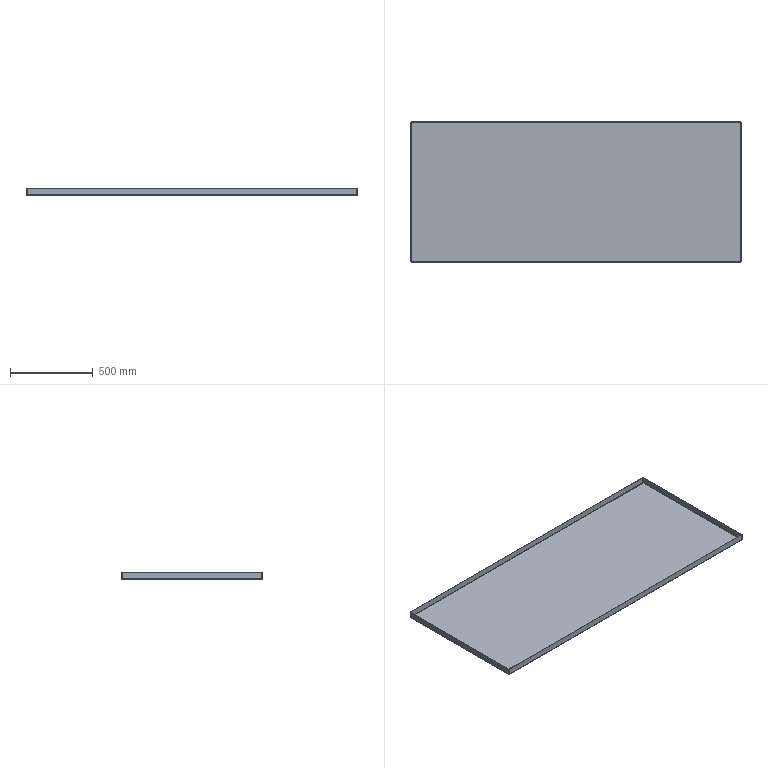Part | SolidWorks | features EdgeFlange 1, FlatPattern 1, SMBaseFlange 1, SheetMetal 1 | 1 solid | 38 faces | box 2000 x 850 x 40 mm | volume 3823030 mm3 | plane 22 | spline 8 | cylinder 8 | commonest cylinder face diameters 1.473 x4 5.473 x4
STEP:
#1=CARTESIAN_POINT('',(997.263,422.263,-2.));
#2=VERTEX_POINT('',#1);
#3=CARTESIAN_POINT('',(997.263,-422.263,-2.));
#4=VERTEX_POINT('',#3);
#5=CARTESIAN_POINT('',(997.263,422.293,-2.));
#6=DIRECTION('',(0.,-1.,0.));
#7=VECTOR('',#6,1000.);
#8=LINE('',#5,#7);
#9=EDGE_CURVE('',#2,#4,#8,.T.);
#10=ORIENTED_EDGE('',*,*,#9,.T.);
#11=CARTESIAN_POINT('',(-997.263,-422.263,-2.));
#12=VERTEX_POINT('',#11);
#13=CARTESIAN_POINT('',(997.293,-422.263,-2.));
#14=DIRECTION('',(-1.,0.,0.));
#15=VECTOR('',#14,1000.);
#16=LINE('',#13,#15);
#17=EDGE_CURVE('',#4,#12,#16,.T.);
#18=ORIENTED_EDGE('',*,*,#17,.T.);
#19=CARTESIAN_POINT('',(-997.263,422.263,-2.));
#20=VERTEX_POINT('',#19);
#21=CARTESIAN_POINT('',(-997.263,-422.293,-2.));
#22=DIRECTION('',(0.,1.,0.));
#23=VECTOR('',#22,1000.);
#24=LINE('',#21,#23);
#25=EDGE_CURVE('',#12,#20,#24,.T.);
#26=ORIENTED_EDGE('',*,*,#25,.T.);
#27=CARTESIAN_POINT('',(-997.293,422.263,-2.));
#28=DIRECTION('',(1.,0.,0.));
#29=VECTOR('',#28,1000.);
#30=LINE('',#27,#29);
#31=EDGE_CURVE('',#20,#2,#30,.T.);
#32=ORIENTED_EDGE('',*,*,#31,.T.);
#33=EDGE_LOOP('',(#10,#18,#26,#32));
#34=FACE_OUTER_BOUND('',#33,.T.);
#35=CARTESIAN_POINT('',(0.,0.,-2.));
#36=DIRECTION('',(0.,0.,-1.));
#37=DIRECTION('',(-1.,0.,0.));
#38=AXIS2_PLACEMENT_3D('',#35,#36,#37);
#39=PLANE('',#38);
#40=ADVANCED_FACE('',(#34),#39,.T.);
#41=CARTESIAN_POINT('',(997.263,-422.263,0.));
#42=VERTEX_POINT('',#41);
#43=CARTESIAN_POINT('',(-997.263,-422.263,0.));
#44=VERTEX_POINT('',#43);
#45=CARTESIAN_POINT('',(997.293,-422.263,0.));
#46=DIRECTION('',(-1.,0.,0.));
#47=VECTOR('',#46,1000.);
#48=LINE('',#45,#47);
#49=EDGE_CURVE('',#42,#44,#48,.T.);
#50=ORIENTED_EDGE('',*,*,#49,.F.);
#51=CARTESIAN_POINT('',(997.263,422.263,0.));
#52=VERTEX_POINT('',#51);
#53=CARTESIAN_POINT('',(997.263,422.293,0.));
#54=DIRECTION('',(0.,-1.,0.));
#55=VECTOR('',#54,1000.);
#56=LINE('',#53,#55);
#57=EDGE_CURVE('',#52,#42,#56,.T.);
#58=ORIENTED_EDGE('',*,*,#57,.F.);
#59=CARTESIAN_POINT('',(-997.263,422.263,0.));
#60=VERTEX_POINT('',#59);
#61=CARTESIAN_POINT('',(-997.293,422.263,0.));
#62=DIRECTION('',(1.,0.,0.));
#63=VECTOR('',#62,1000.);
#64=LINE('',#61,#63);
#65=EDGE_CURVE('',#60,#52,#64,.T.);
#66=ORIENTED_EDGE('',*,*,#65,.F.);
#67=CARTESIAN_POINT('',(-997.263,-422.293,0.));
#68=DIRECTION('',(0.,1.,0.));
#69=VECTOR('',#68,1000.);
#70=LINE('',#67,#69);
#71=EDGE_CURVE('',#44,#60,#70,.T.);
#72=ORIENTED_EDGE('',*,*,#71,.F.);
#73=EDGE_LOOP('',(#50,#58,#66,#72));
#74=FACE_OUTER_BOUND('',#73,.T.);
#75=CARTESIAN_POINT('',(0.,0.,0.));
#76=DIRECTION('',(0.,0.,-1.));
#77=DIRECTION('',(-1.,0.,0.));
#78=AXIS2_PLACEMENT_3D('',#75,#76,#77);
#79=PLANE('',#78);
#80=ADVANCED_FACE('',(#74),#79,.F.);
#81=CARTESIAN_POINT('',(997.293,425.,0.7366));
#82=VERTEX_POINT('',#81);
#83=CARTESIAN_POINT('',(997.293,423.,0.7366));
#84=VERTEX_POINT('',#83);
#85=CARTESIAN_POINT('',(997.293,423.,0.7366));
#86=DIRECTION('',(0.,-1.,0.));
#87=VECTOR('',#86,1000.);
#88=LINE('',#85,#87);
#89=EDGE_CURVE('',#82,#84,#88,.T.);
#90=ORIENTED_EDGE('',*,*,#89,.T.);
#91=CARTESIAN_POINT('',(997.263,422.263,0.));
#92=CARTESIAN_POINT('',(997.268,422.456,0.));
#93=CARTESIAN_POINT('',(997.273,422.648,0.07939));
#94=CARTESIAN_POINT('',(997.283,422.921,0.3521));
#95=CARTESIAN_POINT('',(997.288,423.,0.5438));
#96=CARTESIAN_POINT('',(997.293,423.,0.7366));
#97=B_SPLINE_CURVE_WITH_KNOTS('',3,(#91,#92,#93,#94,#95,#96),.UNSPECIFIED.,.F.,.F.,(4,2,4),(0.,0.5,1.),.UNSPECIFIED.);
#98=EDGE_CURVE('',#52,#84,#97,.T.);
#99=ORIENTED_EDGE('',*,*,#98,.F.);
#100=CARTESIAN_POINT('',(997.263,422.263,0.));
#101=DIRECTION('',(0.,0.,-1.));
#102=VECTOR('',#101,1000.);
#103=LINE('',#100,#102);
#104=EDGE_CURVE('',#52,#2,#103,.T.);
#105=ORIENTED_EDGE('',*,*,#104,.T.);
#106=CARTESIAN_POINT('',(997.263,422.263,-2.));
#107=CARTESIAN_POINT('',(997.266,422.622,-2.));
#108=CARTESIAN_POINT('',(997.268,422.98,-1.929));
#109=CARTESIAN_POINT('',(997.273,423.642,-1.655));
#110=CARTESIAN_POINT('',(997.276,423.945,-1.452));
#111=CARTESIAN_POINT('',(997.281,424.452,-0.9452));
#112=CARTESIAN_POINT('',(997.283,424.655,-0.6416));
#113=CARTESIAN_POINT('',(997.288,424.929,0.0203));
#114=CARTESIAN_POINT('',(997.29,425.,0.3784));
#115=CARTESIAN_POINT('',(997.293,425.,0.7366));
#116=B_SPLINE_CURVE_WITH_KNOTS('',3,(#106,#107,#108,#109,#110,#111,#112,#113,#114,#115),.UNSPECIFIED.,.F.,.F.,(4,2,2,2,4),(0.,0.25,0.5,0.75,1.),.UNSPECIFIED.);
#117=EDGE_CURVE('',#2,#82,#116,.T.);
#118=ORIENTED_EDGE('',*,*,#117,.T.);
#119=EDGE_LOOP('',(#90,#99,#105,#118));
#120=FACE_OUTER_BOUND('',#119,.T.);
#121=CARTESIAN_POINT('',(997.263,422.263,-2.02));
#122=CARTESIAN_POINT('',(997.266,422.624,-2.02));
#123=CARTESIAN_POINT('',(997.268,422.985,-1.948));
#124=CARTESIAN_POINT('',(997.273,423.652,-1.672));
#125=CARTESIAN_POINT('',(997.276,423.957,-1.468));
#126=CARTESIAN_POINT('',(997.281,424.468,-0.9575));
#127=CARTESIAN_POINT('',(997.283,424.672,-0.6517));
#128=CARTESIAN_POINT('',(997.288,424.948,0.01507));
#129=CARTESIAN_POINT('',(997.29,425.02,0.3757));
#130=CARTESIAN_POINT('',(997.293,425.02,0.7366));
#131=CARTESIAN_POINT('',(997.263,422.263,-2.));
#132=CARTESIAN_POINT('',(997.266,422.622,-2.));
#133=CARTESIAN_POINT('',(997.268,422.98,-1.929));
#134=CARTESIAN_POINT('',(997.273,423.642,-1.655));
#135=CARTESIAN_POINT('',(997.276,423.945,-1.452));
#136=CARTESIAN_POINT('',(997.281,424.452,-0.9452));
#137=CARTESIAN_POINT('',(997.283,424.655,-0.6416));
#138=CARTESIAN_POINT('',(997.288,424.929,0.0203));
#139=CARTESIAN_POINT('',(997.29,425.,0.3783));
#140=CARTESIAN_POINT('',(997.293,425.,0.7366));
#141=CARTESIAN_POINT('',(997.263,422.263,0.));
#142=CARTESIAN_POINT('',(997.266,422.36,0.));
#143=CARTESIAN_POINT('',(997.268,422.456,0.01917));
#144=CARTESIAN_POINT('',(997.273,422.634,0.09297));
#145=CARTESIAN_POINT('',(997.276,422.716,0.1476));
#146=CARTESIAN_POINT('',(997.281,422.852,0.2839));
#147=CARTESIAN_POINT('',(997.283,422.907,0.3656));
#148=CARTESIAN_POINT('',(997.288,422.981,0.5438));
#149=CARTESIAN_POINT('',(997.29,423.,0.6402));
#150=CARTESIAN_POINT('',(997.293,423.,0.7366));
#151=CARTESIAN_POINT('',(997.263,422.263,0.0202));
#152=CARTESIAN_POINT('',(997.266,422.357,0.0202));
#153=CARTESIAN_POINT('',(997.268,422.451,0.03885));
#154=CARTESIAN_POINT('',(997.273,422.624,0.1106));
#155=CARTESIAN_POINT('',(997.276,422.704,0.1637));
#156=CARTESIAN_POINT('',(997.281,422.836,0.2963));
#157=CARTESIAN_POINT('',(997.283,422.889,0.3758));
#158=CARTESIAN_POINT('',(997.288,422.961,0.5491));
#159=CARTESIAN_POINT('',(997.29,422.98,0.6428));
#160=CARTESIAN_POINT('',(997.293,422.98,0.7366));
#161=B_SPLINE_SURFACE_WITH_KNOTS('',1,3,((#121,#122,#123,#124,#125,#126,#127,#128,#129,#130),(#131,#132,#133,#134,#135,#136,#137,#138,#139,#140),(#141,#142,#143,#144,#145,#146,#147,#148,#149,#150),(#151,#152,#153,#154,#155,#156,#157,#158,#159,#160)),.UNSPECIFIED.,.F.,.F.,.F.,(2,1,1,2),(4,2,2,2,4),(-0.01,0.,1.,1.01),(0.,0.25,0.5,0.75,1.),.UNSPECIFIED.);
#162=ADVANCED_FACE('',(#120),#161,.F.);
#163=CARTESIAN_POINT('',(-997.293,423.,0.7366));
#164=VERTEX_POINT('',#163);
#165=CARTESIAN_POINT('',(-997.293,423.,0.7366));
#166=CARTESIAN_POINT('',(-997.288,423.,0.5438));
#167=CARTESIAN_POINT('',(-997.283,422.921,0.3521));
#168=CARTESIAN_POINT('',(-997.273,422.648,0.07939));
#169=CARTESIAN_POINT('',(-997.268,422.456,0.));
#170=CARTESIAN_POINT('',(-997.263,422.263,0.));
#171=B_SPLINE_CURVE_WITH_KNOTS('',3,(#165,#166,#167,#168,#169,#170),.UNSPECIFIED.,.F.,.F.,(4,2,4),(0.,0.5,1.),.UNSPECIFIED.);
#172=EDGE_CURVE('',#164,#60,#171,.T.);
#173=ORIENTED_EDGE('',*,*,#172,.F.);
#174=CARTESIAN_POINT('',(-997.293,425.,0.7366));
#175=VERTEX_POINT('',#174);
#176=CARTESIAN_POINT('',(-997.293,423.,0.7366));
#177=DIRECTION('',(0.,-1.,0.));
#178=VECTOR('',#177,1000.);
#179=LINE('',#176,#178);
#180=EDGE_CURVE('',#175,#164,#179,.T.);
#181=ORIENTED_EDGE('',*,*,#180,.F.);
#182=CARTESIAN_POINT('',(-997.293,425.,0.7366));
#183=CARTESIAN_POINT('',(-997.29,425.,0.3784));
#184=CARTESIAN_POINT('',(-997.288,424.929,0.0203));
#185=CARTESIAN_POINT('',(-997.283,424.655,-0.6416));
#186=CARTESIAN_POINT('',(-997.281,424.452,-0.9452));
#187=CARTESIAN_POINT('',(-997.276,423.945,-1.452));
#188=CARTESIAN_POINT('',(-997.273,423.642,-1.655));
#189=CARTESIAN_POINT('',(-997.268,422.98,-1.929));
#190=CARTESIAN_POINT('',(-997.266,422.622,-2.));
#191=CARTESIAN_POINT('',(-997.263,422.263,-2.));
#192=B_SPLINE_CURVE_WITH_KNOTS('',3,(#182,#183,#184,#185,#186,#187,#188,#189,#190,#191),.UNSPECIFIED.,.F.,.F.,(4,2,2,2,4),(0.,0.25,0.5,0.75,1.),.UNSPECIFIED.);
#193=EDGE_CURVE('',#175,#20,#192,.T.);
#194=ORIENTED_EDGE('',*,*,#193,.T.);
#195=CARTESIAN_POINT('',(-997.263,422.263,0.));
#196=DIRECTION('',(0.,0.,-1.));
#197=VECTOR('',#196,1000.);
#198=LINE('',#195,#197);
#199=EDGE_CURVE('',#60,#20,#198,.T.);
#200=ORIENTED_EDGE('',*,*,#199,.F.);
#201=EDGE_LOOP('',(#173,#181,#194,#200));
#202=FACE_OUTER_BOUND('',#201,.T.);
#203=CARTESIAN_POINT('',(-997.293,425.02,0.7366));
#204=CARTESIAN_POINT('',(-997.29,425.02,0.3757));
#205=CARTESIAN_POINT('',(-997.288,424.948,0.01507));
#206=CARTESIAN_POINT('',(-997.283,424.672,-0.6517));
#207=CARTESIAN_POINT('',(-997.281,424.468,-0.9575));
#208=CARTESIAN_POINT('',(-997.276,423.957,-1.468));
#209=CARTESIAN_POINT('',(-997.273,423.652,-1.672));
#210=CARTESIAN_POINT('',(-997.268,422.985,-1.948));
#211=CARTESIAN_POINT('',(-997.266,422.624,-2.02));
#212=CARTESIAN_POINT('',(-997.263,422.263,-2.02));
#213=CARTESIAN_POINT('',(-997.293,425.,0.7366));
#214=CARTESIAN_POINT('',(-997.29,425.,0.3783));
#215=CARTESIAN_POINT('',(-997.288,424.929,0.0203));
#216=CARTESIAN_POINT('',(-997.283,424.655,-0.6416));
#217=CARTESIAN_POINT('',(-997.281,424.452,-0.9452));
#218=CARTESIAN_POINT('',(-997.276,423.945,-1.452));
#219=CARTESIAN_POINT('',(-997.273,423.642,-1.655));
#220=CARTESIAN_POINT('',(-997.268,422.98,-1.929));
#221=CARTESIAN_POINT('',(-997.266,422.622,-2.));
#222=CARTESIAN_POINT('',(-997.263,422.263,-2.));
#223=CARTESIAN_POINT('',(-997.293,423.,0.7366));
#224=CARTESIAN_POINT('',(-997.29,423.,0.6402));
#225=CARTESIAN_POINT('',(-997.288,422.981,0.5438));
#226=CARTESIAN_POINT('',(-997.283,422.907,0.3656));
#227=CARTESIAN_POINT('',(-997.281,422.852,0.2839));
#228=CARTESIAN_POINT('',(-997.276,422.716,0.1476));
#229=CARTESIAN_POINT('',(-997.273,422.634,0.09297));
#230=CARTESIAN_POINT('',(-997.268,422.456,0.01917));
#231=CARTESIAN_POINT('',(-997.266,422.36,0.));
#232=CARTESIAN_POINT('',(-997.263,422.263,0.));
#233=CARTESIAN_POINT('',(-997.293,422.98,0.7366));
#234=CARTESIAN_POINT('',(-997.29,422.98,0.6428));
#235=CARTESIAN_POINT('',(-997.288,422.961,0.5491));
#236=CARTESIAN_POINT('',(-997.283,422.889,0.3758));
#237=CARTESIAN_POINT('',(-997.281,422.836,0.2963));
#238=CARTESIAN_POINT('',(-997.276,422.704,0.1637));
#239=CARTESIAN_POINT('',(-997.273,422.624,0.1106));
#240=CARTESIAN_POINT('',(-997.268,422.451,0.03885));
#241=CARTESIAN_POINT('',(-997.266,422.357,0.0202));
#242=CARTESIAN_POINT('',(-997.263,422.263,0.0202));
#243=B_SPLINE_SURFACE_WITH_KNOTS('',1,3,((#203,#204,#205,#206,#207,#208,#209,#210,#211,#212),(#213,#214,#215,#216,#217,#218,#219,#220,#221,#222),(#223,#224,#225,#226,#227,#228,#229,#230,#231,#232),(#233,#234,#235,#236,#237,#238,#239,#240,#241,#242)),.UNSPECIFIED.,.F.,.F.,.F.,(2,1,1,2),(4,2,2,2,4),(-0.01,0.,1.,1.01),(0.,0.25,0.5,0.75,1.),.UNSPECIFIED.);
#244=ADVANCED_FACE('',(#202),#243,.F.);
#245=ORIENTED_EDGE('',*,*,#31,.F.);
#246=ORIENTED_EDGE('',*,*,#193,.F.);
#247=CARTESIAN_POINT('',(0.,425.,0.7366));
#248=DIRECTION('',(-1.,0.,0.));
#249=VECTOR('',#248,1000.);
#250=LINE('',#247,#249);
#251=EDGE_CURVE('',#82,#175,#250,.T.);
#252=ORIENTED_EDGE('',*,*,#251,.F.);
#253=ORIENTED_EDGE('',*,*,#117,.F.);
#254=EDGE_LOOP('',(#245,#246,#252,#253));
#255=FACE_OUTER_BOUND('',#254,.T.);
#256=CARTESIAN_POINT('',(-997.293,422.263,0.7366));
#257=DIRECTION('',(-1.,0.,0.));
#258=DIRECTION('',(0.,1.,0.));
#259=AXIS2_PLACEMENT_3D('',#256,#257,#258);
#260=CYLINDRICAL_SURFACE('',#259,2.737);
#261=ADVANCED_FACE('',(#255),#260,.T.);
#262=ORIENTED_EDGE('',*,*,#65,.T.);
#263=ORIENTED_EDGE('',*,*,#98,.T.);
#264=CARTESIAN_POINT('',(1000.,423.,0.7366));
#265=DIRECTION('',(-1.,0.,0.));
#266=VECTOR('',#265,1000.);
#267=LINE('',#264,#266);
#268=EDGE_CURVE('',#84,#164,#267,.T.);
#269=ORIENTED_EDGE('',*,*,#268,.T.);
#270=ORIENTED_EDGE('',*,*,#172,.T.);
#271=EDGE_LOOP('',(#262,#263,#269,#270));
#272=FACE_OUTER_BOUND('',#271,.T.);
#273=CARTESIAN_POINT('',(-997.293,422.263,0.7366));
#274=DIRECTION('',(-1.,0.,0.));
#275=DIRECTION('',(0.,1.,0.));
#276=AXIS2_PLACEMENT_3D('',#273,#274,#275);
#277=CYLINDRICAL_SURFACE('',#276,0.7366);
#278=ADVANCED_FACE('',(#272),#277,.F.);
#279=CARTESIAN_POINT('',(997.293,423.,38.));
#280=VERTEX_POINT('',#279);
#281=CARTESIAN_POINT('',(997.293,425.,38.));
#282=VERTEX_POINT('',#281);
#283=CARTESIAN_POINT('',(997.293,425.,38.));
#284=DIRECTION('',(0.,1.,0.));
#285=VECTOR('',#284,1000.);
#286=LINE('',#283,#285);
#287=EDGE_CURVE('',#280,#282,#286,.T.);
#288=ORIENTED_EDGE('',*,*,#287,.F.);
#289=CARTESIAN_POINT('',(997.293,423.,0.));
#290=DIRECTION('',(0.,0.,1.));
#291=VECTOR('',#290,1000.);
#292=LINE('',#289,#291);
#293=EDGE_CURVE('',#84,#280,#292,.T.);
#294=ORIENTED_EDGE('',*,*,#293,.F.);
#295=ORIENTED_EDGE('',*,*,#89,.F.);
#296=CARTESIAN_POINT('',(997.293,425.,0.));
#297=DIRECTION('',(0.,0.,-1.));
#298=VECTOR('',#297,1000.);
#299=LINE('',#296,#298);
#300=EDGE_CURVE('',#282,#82,#299,.T.);
#301=ORIENTED_EDGE('',*,*,#300,.F.);
#302=EDGE_LOOP('',(#288,#294,#295,#301));
#303=FACE_OUTER_BOUND('',#302,.T.);
#304=CARTESIAN_POINT('',(997.293,423.,0.));
#305=DIRECTION('',(1.,0.,0.));
#306=DIRECTION('',(0.,0.,-1.));
#307=AXIS2_PLACEMENT_3D('',#304,#305,#306);
#308=PLANE('',#307);
#309=ADVANCED_FACE('',(#303),#308,.T.);
#310=CARTESIAN_POINT('',(-997.293,425.,38.));
#311=VERTEX_POINT('',#310);
#312=CARTESIAN_POINT('',(-997.293,425.,0.));
#313=DIRECTION('',(0.,0.,-1.));
#314=VECTOR('',#313,1000.);
#315=LINE('',#312,#314);
#316=EDGE_CURVE('',#311,#175,#315,.T.);
#317=ORIENTED_EDGE('',*,*,#316,.F.);
#318=CARTESIAN_POINT('',(-1000.,425.,38.));
#319=DIRECTION('',(-1.,0.,0.));
#320=VECTOR('',#319,1000.);
#321=LINE('',#318,#320);
#322=EDGE_CURVE('',#282,#311,#321,.T.);
#323=ORIENTED_EDGE('',*,*,#322,.F.);
#324=ORIENTED_EDGE('',*,*,#300,.T.);
#325=ORIENTED_EDGE('',*,*,#251,.T.);
#326=EDGE_LOOP('',(#317,#323,#324,#325));
#327=FACE_OUTER_BOUND('',#326,.T.);
#328=CARTESIAN_POINT('',(0.,425.,0.));
#329=DIRECTION('',(0.,1.,0.));
#330=DIRECTION('',(0.,0.,1.));
#331=AXIS2_PLACEMENT_3D('',#328,#329,#330);
#332=PLANE('',#331);
#333=ADVANCED_FACE('',(#327),#332,.T.);
#334=CARTESIAN_POINT('',(-997.293,423.,38.));
#335=VERTEX_POINT('',#334);
#336=CARTESIAN_POINT('',(0.,423.,38.));
#337=DIRECTION('',(-1.,0.,0.));
#338=VECTOR('',#337,1000.);
#339=LINE('',#336,#338);
#340=EDGE_CURVE('',#280,#335,#339,.T.);
#341=ORIENTED_EDGE('',*,*,#340,.T.);
#342=CARTESIAN_POINT('',(-997.293,423.,0.));
#343=DIRECTION('',(0.,0.,1.));
#344=VECTOR('',#343,1000.);
#345=LINE('',#342,#344);
#346=EDGE_CURVE('',#164,#335,#345,.T.);
#347=ORIENTED_EDGE('',*,*,#346,.F.);
#348=ORIENTED_EDGE('',*,*,#268,.F.);
#349=ORIENTED_EDGE('',*,*,#293,.T.);
#350=EDGE_LOOP('',(#341,#347,#348,#349));
#351=FACE_OUTER_BOUND('',#350,.T.);
#352=CARTESIAN_POINT('',(0.,423.,0.));
#353=DIRECTION('',(0.,1.,0.));
#354=DIRECTION('',(0.,0.,1.));
#355=AXIS2_PLACEMENT_3D('',#352,#353,#354);
#356=PLANE('',#355);
#357=ADVANCED_FACE('',(#351),#356,.F.);
#358=CARTESIAN_POINT('',(-997.293,423.,38.));
#359=DIRECTION('',(0.,1.,0.));
#360=VECTOR('',#359,1000.);
#361=LINE('',#358,#360);
#362=EDGE_CURVE('',#335,#311,#361,.T.);
#363=ORIENTED_EDGE('',*,*,#362,.F.);
#364=ORIENTED_EDGE('',*,*,#340,.F.);
#365=ORIENTED_EDGE('',*,*,#287,.T.);
#366=ORIENTED_EDGE('',*,*,#322,.T.);
#367=EDGE_LOOP('',(#363,#364,#365,#366));
#368=FACE_OUTER_BOUND('',#367,.T.);
#369=CARTESIAN_POINT('',(-1000.,425.,38.));
#370=DIRECTION('',(0.,0.,1.));
#371=DIRECTION('',(0.,-1.,0.));
#372=AXIS2_PLACEMENT_3D('',#369,#370,#371);
#373=PLANE('',#372);
#374=ADVANCED_FACE('',(#368),#373,.T.);
#375=ORIENTED_EDGE('',*,*,#346,.T.);
#376=ORIENTED_EDGE('',*,*,#362,.T.);
#377=ORIENTED_EDGE('',*,*,#316,.T.);
#378=ORIENTED_EDGE('',*,*,#180,.T.);
#379=EDGE_LOOP('',(#375,#376,#377,#378));
#380=FACE_OUTER_BOUND('',#379,.T.);
#381=CARTESIAN_POINT('',(-997.293,423.,0.));
#382=DIRECTION('',(1.,0.,0.));
#383=DIRECTION('',(0.,0.,-1.));
#384=AXIS2_PLACEMENT_3D('',#381,#382,#383);
#385=PLANE('',#384);
#386=ADVANCED_FACE('',(#380),#385,.F.);
#387=CARTESIAN_POINT('',(-1000.,422.293,0.7366));
#388=VERTEX_POINT('',#387);
#389=CARTESIAN_POINT('',(-998.,422.293,0.7366));
#390=VERTEX_POINT('',#389);
#391=CARTESIAN_POINT('',(-998.,422.293,0.7366));
#392=DIRECTION('',(1.,0.,0.));
#393=VECTOR('',#392,1000.);
#394=LINE('',#391,#393);
#395=EDGE_CURVE('',#388,#390,#394,.T.);
#396=ORIENTED_EDGE('',*,*,#395,.T.);
#397=CARTESIAN_POINT('',(-997.263,422.263,0.));
#398=CARTESIAN_POINT('',(-997.456,422.268,0.));
#399=CARTESIAN_POINT('',(-997.648,422.273,0.07939));
#400=CARTESIAN_POINT('',(-997.921,422.283,0.3521));
#401=CARTESIAN_POINT('',(-998.,422.288,0.5438));
#402=CARTESIAN_POINT('',(-998.,422.293,0.7366));
#403=B_SPLINE_CURVE_WITH_KNOTS('',3,(#397,#398,#399,#400,#401,#402),.UNSPECIFIED.,.F.,.F.,(4,2,4),(0.,0.5,1.),.UNSPECIFIED.);
#404=EDGE_CURVE('',#60,#390,#403,.T.);
#405=ORIENTED_EDGE('',*,*,#404,.F.);
#406=ORIENTED_EDGE('',*,*,#199,.T.);
#407=CARTESIAN_POINT('',(-997.263,422.263,-2.));
#408=CARTESIAN_POINT('',(-997.622,422.266,-2.));
#409=CARTESIAN_POINT('',(-997.98,422.268,-1.929));
#410=CARTESIAN_POINT('',(-998.642,422.273,-1.655));
#411=CARTESIAN_POINT('',(-998.945,422.276,-1.452));
#412=CARTESIAN_POINT('',(-999.452,422.281,-0.9452));
#413=CARTESIAN_POINT('',(-999.655,422.283,-0.6416));
#414=CARTESIAN_POINT('',(-999.929,422.288,0.0203));
#415=CARTESIAN_POINT('',(-1000.,422.29,0.3784));
#416=CARTESIAN_POINT('',(-1000.,422.293,0.7366));
#417=B_SPLINE_CURVE_WITH_KNOTS('',3,(#407,#408,#409,#410,#411,#412,#413,#414,#415,#416),.UNSPECIFIED.,.F.,.F.,(4,2,2,2,4),(0.,0.25,0.5,0.75,1.),.UNSPECIFIED.);
#418=EDGE_CURVE('',#20,#388,#417,.T.);
#419=ORIENTED_EDGE('',*,*,#418,.T.);
#420=EDGE_LOOP('',(#396,#405,#406,#419));
#421=FACE_OUTER_BOUND('',#420,.T.);
#422=CARTESIAN_POINT('',(-997.263,422.263,-2.02));
#423=CARTESIAN_POINT('',(-997.624,422.266,-2.02));
#424=CARTESIAN_POINT('',(-997.985,422.268,-1.948));
#425=CARTESIAN_POINT('',(-998.652,422.273,-1.672));
#426=CARTESIAN_POINT('',(-998.957,422.276,-1.468));
#427=CARTESIAN_POINT('',(-999.468,422.281,-0.9575));
#428=CARTESIAN_POINT('',(-999.672,422.283,-0.6517));
#429=CARTESIAN_POINT('',(-999.948,422.288,0.01507));
#430=CARTESIAN_POINT('',(-1000.02,422.29,0.3757));
#431=CARTESIAN_POINT('',(-1000.02,422.293,0.7366));
#432=CARTESIAN_POINT('',(-997.263,422.263,-2.));
#433=CARTESIAN_POINT('',(-997.622,422.266,-2.));
#434=CARTESIAN_POINT('',(-997.98,422.268,-1.929));
#435=CARTESIAN_POINT('',(-998.642,422.273,-1.655));
#436=CARTESIAN_POINT('',(-998.945,422.276,-1.452));
#437=CARTESIAN_POINT('',(-999.452,422.281,-0.9452));
#438=CARTESIAN_POINT('',(-999.655,422.283,-0.6416));
#439=CARTESIAN_POINT('',(-999.929,422.288,0.0203));
#440=CARTESIAN_POINT('',(-1000.,422.29,0.3783));
#441=CARTESIAN_POINT('',(-1000.,422.293,0.7366));
#442=CARTESIAN_POINT('',(-997.263,422.263,0.));
#443=CARTESIAN_POINT('',(-997.36,422.266,0.));
#444=CARTESIAN_POINT('',(-997.456,422.268,0.01917));
#445=CARTESIAN_POINT('',(-997.634,422.273,0.09297));
#446=CARTESIAN_POINT('',(-997.716,422.276,0.1476));
#447=CARTESIAN_POINT('',(-997.852,422.281,0.2839));
#448=CARTESIAN_POINT('',(-997.907,422.283,0.3656));
#449=CARTESIAN_POINT('',(-997.981,422.288,0.5438));
#450=CARTESIAN_POINT('',(-998.,422.29,0.6402));
#451=CARTESIAN_POINT('',(-998.,422.293,0.7366));
#452=CARTESIAN_POINT('',(-997.263,422.263,0.0202));
#453=CARTESIAN_POINT('',(-997.357,422.266,0.0202));
#454=CARTESIAN_POINT('',(-997.451,422.268,0.03885));
#455=CARTESIAN_POINT('',(-997.624,422.273,0.1106));
#456=CARTESIAN_POINT('',(-997.704,422.276,0.1637));
#457=CARTESIAN_POINT('',(-997.836,422.281,0.2963));
#458=CARTESIAN_POINT('',(-997.889,422.283,0.3758));
#459=CARTESIAN_POINT('',(-997.961,422.288,0.5491));
#460=CARTESIAN_POINT('',(-997.98,422.29,0.6428));
#461=CARTESIAN_POINT('',(-997.98,422.293,0.7366));
#462=B_SPLINE_SURFACE_WITH_KNOTS('',1,3,((#422,#423,#424,#425,#426,#427,#428,#429,#430,#431),(#432,#433,#434,#435,#436,#437,#438,#439,#440,#441),(#442,#443,#444,#445,#446,#447,#448,#449,#450,#451),(#452,#453,#454,#455,#456,#457,#458,#459,#460,#461)),.UNSPECIFIED.,.F.,.F.,.F.,(2,1,1,2),(4,2,2,2,4),(-0.01,0.,1.,1.01),(0.,0.25,0.5,0.75,1.),.UNSPECIFIED.);
#463=ADVANCED_FACE('',(#421),#462,.F.);
#464=CARTESIAN_POINT('',(-998.,-422.293,0.7366));
#465=VERTEX_POINT('',#464);
#466=CARTESIAN_POINT('',(-998.,-422.293,0.7366));
#467=CARTESIAN_POINT('',(-998.,-422.288,0.5438));
#468=CARTESIAN_POINT('',(-997.921,-422.283,0.3521));
#469=CARTESIAN_POINT('',(-997.648,-422.273,0.07939));
#470=CARTESIAN_POINT('',(-997.456,-422.268,0.));
#471=CARTESIAN_POINT('',(-997.263,-422.263,0.));
#472=B_SPLINE_CURVE_WITH_KNOTS('',3,(#466,#467,#468,#469,#470,#471),.UNSPECIFIED.,.F.,.F.,(4,2,4),(0.,0.5,1.),.UNSPECIFIED.);
#473=EDGE_CURVE('',#465,#44,#472,.T.);
#474=ORIENTED_EDGE('',*,*,#473,.F.);
#475=CARTESIAN_POINT('',(-1000.,-422.293,0.7366));
#476=VERTEX_POINT('',#475);
#477=CARTESIAN_POINT('',(-998.,-422.293,0.7366));
#478=DIRECTION('',(1.,0.,0.));
#479=VECTOR('',#478,1000.);
#480=LINE('',#477,#479);
#481=EDGE_CURVE('',#476,#465,#480,.T.);
#482=ORIENTED_EDGE('',*,*,#481,.F.);
#483=CARTESIAN_POINT('',(-1000.,-422.293,0.7366));
#484=CARTESIAN_POINT('',(-1000.,-422.29,0.3784));
#485=CARTESIAN_POINT('',(-999.929,-422.288,0.0203));
#486=CARTESIAN_POINT('',(-999.655,-422.283,-0.6416));
#487=CARTESIAN_POINT('',(-999.452,-422.281,-0.9452));
#488=CARTESIAN_POINT('',(-998.945,-422.276,-1.452));
#489=CARTESIAN_POINT('',(-998.642,-422.273,-1.655));
#490=CARTESIAN_POINT('',(-997.98,-422.268,-1.929));
#491=CARTESIAN_POINT('',(-997.622,-422.266,-2.));
#492=CARTESIAN_POINT('',(-997.263,-422.263,-2.));
#493=B_SPLINE_CURVE_WITH_KNOTS('',3,(#483,#484,#485,#486,#487,#488,#489,#490,#491,#492),.UNSPECIFIED.,.F.,.F.,(4,2,2,2,4),(0.,0.25,0.5,0.75,1.),.UNSPECIFIED.);
#494=EDGE_CURVE('',#476,#12,#493,.T.);
#495=ORIENTED_EDGE('',*,*,#494,.T.);
#496=CARTESIAN_POINT('',(-997.263,-422.263,0.));
#497=DIRECTION('',(0.,0.,-1.));
#498=VECTOR('',#497,1000.);
#499=LINE('',#496,#498);
#500=EDGE_CURVE('',#44,#12,#499,.T.);
#501=ORIENTED_EDGE('',*,*,#500,.F.);
#502=EDGE_LOOP('',(#474,#482,#495,#501));
#503=FACE_OUTER_BOUND('',#502,.T.);
#504=CARTESIAN_POINT('',(-1000.02,-422.293,0.7366));
#505=CARTESIAN_POINT('',(-1000.02,-422.29,0.3757));
#506=CARTESIAN_POINT('',(-999.948,-422.288,0.01507));
#507=CARTESIAN_POINT('',(-999.672,-422.283,-0.6517));
#508=CARTESIAN_POINT('',(-999.468,-422.281,-0.9575));
#509=CARTESIAN_POINT('',(-998.957,-422.276,-1.468));
#510=CARTESIAN_POINT('',(-998.652,-422.273,-1.672));
#511=CARTESIAN_POINT('',(-997.985,-422.268,-1.948));
#512=CARTESIAN_POINT('',(-997.624,-422.266,-2.02));
#513=CARTESIAN_POINT('',(-997.263,-422.263,-2.02));
#514=CARTESIAN_POINT('',(-1000.,-422.293,0.7366));
#515=CARTESIAN_POINT('',(-1000.,-422.29,0.3783));
#516=CARTESIAN_POINT('',(-999.929,-422.288,0.0203));
#517=CARTESIAN_POINT('',(-999.655,-422.283,-0.6416));
#518=CARTESIAN_POINT('',(-999.452,-422.281,-0.9452));
#519=CARTESIAN_POINT('',(-998.945,-422.276,-1.452));
#520=CARTESIAN_POINT('',(-998.642,-422.273,-1.655));
#521=CARTESIAN_POINT('',(-997.98,-422.268,-1.929));
#522=CARTESIAN_POINT('',(-997.622,-422.266,-2.));
#523=CARTESIAN_POINT('',(-997.263,-422.263,-2.));
#524=CARTESIAN_POINT('',(-998.,-422.293,0.7366));
#525=CARTESIAN_POINT('',(-998.,-422.29,0.6402));
#526=CARTESIAN_POINT('',(-997.981,-422.288,0.5438));
#527=CARTESIAN_POINT('',(-997.907,-422.283,0.3656));
#528=CARTESIAN_POINT('',(-997.852,-422.281,0.2839));
#529=CARTESIAN_POINT('',(-997.716,-422.276,0.1476));
#530=CARTESIAN_POINT('',(-997.634,-422.273,0.09297));
#531=CARTESIAN_POINT('',(-997.456,-422.268,0.01917));
#532=CARTESIAN_POINT('',(-997.36,-422.266,0.));
#533=CARTESIAN_POINT('',(-997.263,-422.263,0.));
#534=CARTESIAN_POINT('',(-997.98,-422.293,0.7366));
#535=CARTESIAN_POINT('',(-997.98,-422.29,0.6428));
#536=CARTESIAN_POINT('',(-997.961,-422.288,0.5491));
#537=CARTESIAN_POINT('',(-997.889,-422.283,0.3758));
#538=CARTESIAN_POINT('',(-997.836,-422.281,0.2963));
#539=CARTESIAN_POINT('',(-997.704,-422.276,0.1637));
#540=CARTESIAN_POINT('',(-997.624,-422.273,0.1106));
#541=CARTESIAN_POINT('',(-997.451,-422.268,0.03885));
#542=CARTESIAN_POINT('',(-997.357,-422.266,0.0202));
#543=CARTESIAN_POINT('',(-997.263,-422.263,0.0202));
#544=B_SPLINE_SURFACE_WITH_KNOTS('',1,3,((#504,#505,#506,#507,#508,#509,#510,#511,#512,#513),(#514,#515,#516,#517,#518,#519,#520,#521,#522,#523),(#524,#525,#526,#527,#528,#529,#530,#531,#532,#533),(#534,#535,#536,#537,#538,#539,#540,#541,#542,#543)),.UNSPECIFIED.,.F.,.F.,.F.,(2,1,1,2),(4,2,2,2,4),(-0.01,0.,1.,1.01),(0.,0.25,0.5,0.75,1.),.UNSPECIFIED.);
#545=ADVANCED_FACE('',(#503),#544,.F.);
#546=ORIENTED_EDGE('',*,*,#25,.F.);
#547=ORIENTED_EDGE('',*,*,#494,.F.);
#548=CARTESIAN_POINT('',(-1000.,425.,0.7366));
#549=DIRECTION('',(0.,1.,0.));
#550=VECTOR('',#549,1000.);
#551=LINE('',#548,#550);
#552=EDGE_CURVE('',#476,#388,#551,.T.);
#553=ORIENTED_EDGE('',*,*,#552,.T.);
#554=ORIENTED_EDGE('',*,*,#418,.F.);
#555=EDGE_LOOP('',(#546,#547,#553,#554));
#556=FACE_OUTER_BOUND('',#555,.T.);
#557=CARTESIAN_POINT('',(-997.263,-422.293,0.7366));
#558=DIRECTION('',(0.,-1.,0.));
#559=DIRECTION('',(-1.,0.,0.));
#560=AXIS2_PLACEMENT_3D('',#557,#558,#559);
#561=CYLINDRICAL_SURFACE('',#560,2.737);
#562=ADVANCED_FACE('',(#556),#561,.T.);
#563=ORIENTED_EDGE('',*,*,#71,.T.);
#564=ORIENTED_EDGE('',*,*,#404,.T.);
#565=CARTESIAN_POINT('',(-998.,425.,0.7366));
#566=DIRECTION('',(0.,-1.,0.));
#567=VECTOR('',#566,1000.);
#568=LINE('',#565,#567);
#569=EDGE_CURVE('',#390,#465,#568,.T.);
#570=ORIENTED_EDGE('',*,*,#569,.T.);
#571=ORIENTED_EDGE('',*,*,#473,.T.);
#572=EDGE_LOOP('',(#563,#564,#570,#571));
#573=FACE_OUTER_BOUND('',#572,.T.);
#574=CARTESIAN_POINT('',(-997.263,-422.293,0.7366));
#575=DIRECTION('',(0.,-1.,0.));
#576=DIRECTION('',(-1.,0.,0.));
#577=AXIS2_PLACEMENT_3D('',#574,#575,#576);
#578=CYLINDRICAL_SURFACE('',#577,0.7366);
#579=ADVANCED_FACE('',(#573),#578,.F.);
#580=CARTESIAN_POINT('',(-998.,422.293,38.));
#581=VERTEX_POINT('',#580);
#582=CARTESIAN_POINT('',(-1000.,422.293,38.));
#583=VERTEX_POINT('',#582);
#584=CARTESIAN_POINT('',(-1000.,422.293,38.));
#585=DIRECTION('',(-1.,0.,0.));
#586=VECTOR('',#585,1000.);
#587=LINE('',#584,#586);
#588=EDGE_CURVE('',#581,#583,#587,.T.);
#589=ORIENTED_EDGE('',*,*,#588,.F.);
#590=CARTESIAN_POINT('',(-998.,422.293,0.));
#591=DIRECTION('',(0.,0.,1.));
#592=VECTOR('',#591,1000.);
#593=LINE('',#590,#592);
#594=EDGE_CURVE('',#390,#581,#593,.T.);
#595=ORIENTED_EDGE('',*,*,#594,.F.);
#596=ORIENTED_EDGE('',*,*,#395,.F.);
#597=CARTESIAN_POINT('',(-1000.,422.293,0.));
#598=DIRECTION('',(0.,0.,1.));
#599=VECTOR('',#598,1000.);
#600=LINE('',#597,#599);
#601=EDGE_CURVE('',#388,#583,#600,.T.);
#602=ORIENTED_EDGE('',*,*,#601,.T.);
#603=EDGE_LOOP('',(#589,#595,#596,#602));
#604=FACE_OUTER_BOUND('',#603,.T.);
#605=CARTESIAN_POINT('',(-998.,422.293,0.));
#606=DIRECTION('',(0.,1.,0.));
#607=DIRECTION('',(0.,0.,1.));
#608=AXIS2_PLACEMENT_3D('',#605,#606,#607);
#609=PLANE('',#608);
#610=ADVANCED_FACE('',(#604),#609,.T.);
#611=ORIENTED_EDGE('',*,*,#552,.F.);
#612=CARTESIAN_POINT('',(-1000.,-422.293,38.));
#613=VERTEX_POINT('',#612);
#614=CARTESIAN_POINT('',(-1000.,-422.293,0.));
#615=DIRECTION('',(0.,0.,1.));
#616=VECTOR('',#615,1000.);
#617=LINE('',#614,#616);
#618=EDGE_CURVE('',#476,#613,#617,.T.);
#619=ORIENTED_EDGE('',*,*,#618,.T.);
#620=CARTESIAN_POINT('',(-1000.,425.,38.));
#621=DIRECTION('',(0.,-1.,0.));
#622=VECTOR('',#621,1000.);
#623=LINE('',#620,#622);
#624=EDGE_CURVE('',#583,#613,#623,.T.);
#625=ORIENTED_EDGE('',*,*,#624,.F.);
#626=ORIENTED_EDGE('',*,*,#601,.F.);
#627=EDGE_LOOP('',(#611,#619,#625,#626));
#628=FACE_OUTER_BOUND('',#627,.T.);
#629=CARTESIAN_POINT('',(-1000.,0.,0.));
#630=DIRECTION('',(1.,0.,0.));
#631=DIRECTION('',(0.,0.,-1.));
#632=AXIS2_PLACEMENT_3D('',#629,#630,#631);
#633=PLANE('',#632);
#634=ADVANCED_FACE('',(#628),#633,.F.);
#635=CARTESIAN_POINT('',(-998.,-422.293,38.));
#636=VERTEX_POINT('',#635);
#637=CARTESIAN_POINT('',(-998.,-422.293,0.));
#638=DIRECTION('',(0.,0.,1.));
#639=VECTOR('',#638,1000.);
#640=LINE('',#637,#639);
#641=EDGE_CURVE('',#465,#636,#640,.T.);
#642=ORIENTED_EDGE('',*,*,#641,.F.);
#643=ORIENTED_EDGE('',*,*,#569,.F.);
#644=ORIENTED_EDGE('',*,*,#594,.T.);
#645=CARTESIAN_POINT('',(-998.,0.,38.));
#646=DIRECTION('',(0.,-1.,0.));
#647=VECTOR('',#646,1000.);
#648=LINE('',#645,#647);
#649=EDGE_CURVE('',#581,#636,#648,.T.);
#650=ORIENTED_EDGE('',*,*,#649,.T.);
#651=EDGE_LOOP('',(#642,#643,#644,#650));
#652=FACE_OUTER_BOUND('',#651,.T.);
#653=CARTESIAN_POINT('',(-998.,0.,0.));
#654=DIRECTION('',(1.,0.,0.));
#655=DIRECTION('',(0.,0.,-1.));
#656=AXIS2_PLACEMENT_3D('',#653,#654,#655);
#657=PLANE('',#656);
#658=ADVANCED_FACE('',(#652),#657,.T.);
#659=CARTESIAN_POINT('',(-998.,-422.293,38.));
#660=DIRECTION('',(-1.,0.,0.));
#661=VECTOR('',#660,1000.);
#662=LINE('',#659,#661);
#663=EDGE_CURVE('',#636,#613,#662,.T.);
#664=ORIENTED_EDGE('',*,*,#663,.F.);
#665=ORIENTED_EDGE('',*,*,#649,.F.);
#666=ORIENTED_EDGE('',*,*,#588,.T.);
#667=ORIENTED_EDGE('',*,*,#624,.T.);
#668=EDGE_LOOP('',(#664,#665,#666,#667));
#669=FACE_OUTER_BOUND('',#668,.T.);
#670=CARTESIAN_POINT('',(-1000.,425.,38.));
#671=DIRECTION('',(0.,0.,1.));
#672=DIRECTION('',(1.,0.,0.));
#673=AXIS2_PLACEMENT_3D('',#670,#671,#672);
#674=PLANE('',#673);
#675=ADVANCED_FACE('',(#669),#674,.T.);
#676=ORIENTED_EDGE('',*,*,#641,.T.);
#677=ORIENTED_EDGE('',*,*,#663,.T.);
#678=ORIENTED_EDGE('',*,*,#618,.F.);
#679=ORIENTED_EDGE('',*,*,#481,.T.);
#680=EDGE_LOOP('',(#676,#677,#678,#679));
#681=FACE_OUTER_BOUND('',#680,.T.);
#682=CARTESIAN_POINT('',(-998.,-422.293,0.));
#683=DIRECTION('',(0.,1.,0.));
#684=DIRECTION('',(0.,0.,1.));
#685=AXIS2_PLACEMENT_3D('',#682,#683,#684);
#686=PLANE('',#685);
#687=ADVANCED_FACE('',(#681),#686,.F.);
#688=CARTESIAN_POINT('',(1000.,-422.293,0.7366));
#689=VERTEX_POINT('',#688);
#690=CARTESIAN_POINT('',(998.,-422.293,0.7366));
#691=VERTEX_POINT('',#690);
#692=CARTESIAN_POINT('',(998.,-422.293,0.7366));
#693=DIRECTION('',(-1.,0.,0.));
#694=VECTOR('',#693,1000.);
#695=LINE('',#692,#694);
#696=EDGE_CURVE('',#689,#691,#695,.T.);
#697=ORIENTED_EDGE('',*,*,#696,.T.);
#698=CARTESIAN_POINT('',(997.263,-422.263,0.));
#699=CARTESIAN_POINT('',(997.456,-422.268,0.));
#700=CARTESIAN_POINT('',(997.648,-422.273,0.07939));
#701=CARTESIAN_POINT('',(997.921,-422.283,0.3521));
#702=CARTESIAN_POINT('',(998.,-422.288,0.5438));
#703=CARTESIAN_POINT('',(998.,-422.293,0.7366));
#704=B_SPLINE_CURVE_WITH_KNOTS('',3,(#698,#699,#700,#701,#702,#703),.UNSPECIFIED.,.F.,.F.,(4,2,4),(0.,0.5,1.),.UNSPECIFIED.);
#705=EDGE_CURVE('',#42,#691,#704,.T.);
#706=ORIENTED_EDGE('',*,*,#705,.F.);
#707=CARTESIAN_POINT('',(997.263,-422.263,0.));
#708=DIRECTION('',(0.,0.,-1.));
#709=VECTOR('',#708,1000.);
#710=LINE('',#707,#709);
#711=EDGE_CURVE('',#42,#4,#710,.T.);
#712=ORIENTED_EDGE('',*,*,#711,.T.);
#713=CARTESIAN_POINT('',(997.263,-422.263,-2.));
#714=CARTESIAN_POINT('',(997.622,-422.266,-2.));
#715=CARTESIAN_POINT('',(997.98,-422.268,-1.929));
#716=CARTESIAN_POINT('',(998.642,-422.273,-1.655));
#717=CARTESIAN_POINT('',(998.945,-422.276,-1.452));
#718=CARTESIAN_POINT('',(999.452,-422.281,-0.9452));
#719=CARTESIAN_POINT('',(999.655,-422.283,-0.6416));
#720=CARTESIAN_POINT('',(999.929,-422.288,0.0203));
#721=CARTESIAN_POINT('',(1000.,-422.29,0.3784));
#722=CARTESIAN_POINT('',(1000.,-422.293,0.7366));
#723=B_SPLINE_CURVE_WITH_KNOTS('',3,(#713,#714,#715,#716,#717,#718,#719,#720,#721,#722),.UNSPECIFIED.,.F.,.F.,(4,2,2,2,4),(0.,0.25,0.5,0.75,1.),.UNSPECIFIED.);
#724=EDGE_CURVE('',#4,#689,#723,.T.);
#725=ORIENTED_EDGE('',*,*,#724,.T.);
#726=EDGE_LOOP('',(#697,#706,#712,#725));
#727=FACE_OUTER_BOUND('',#726,.T.);
#728=CARTESIAN_POINT('',(997.263,-422.263,-2.02));
#729=CARTESIAN_POINT('',(997.624,-422.266,-2.02));
#730=CARTESIAN_POINT('',(997.985,-422.268,-1.948));
#731=CARTESIAN_POINT('',(998.652,-422.273,-1.672));
#732=CARTESIAN_POINT('',(998.957,-422.276,-1.468));
#733=CARTESIAN_POINT('',(999.468,-422.281,-0.9575));
#734=CARTESIAN_POINT('',(999.672,-422.283,-0.6517));
#735=CARTESIAN_POINT('',(999.948,-422.288,0.01507));
#736=CARTESIAN_POINT('',(1000.02,-422.29,0.3757));
#737=CARTESIAN_POINT('',(1000.02,-422.293,0.7366));
#738=CARTESIAN_POINT('',(997.263,-422.263,-2.));
#739=CARTESIAN_POINT('',(997.622,-422.266,-2.));
#740=CARTESIAN_POINT('',(997.98,-422.268,-1.929));
#741=CARTESIAN_POINT('',(998.642,-422.273,-1.655));
#742=CARTESIAN_POINT('',(998.945,-422.276,-1.452));
#743=CARTESIAN_POINT('',(999.452,-422.281,-0.9452));
#744=CARTESIAN_POINT('',(999.655,-422.283,-0.6416));
#745=CARTESIAN_POINT('',(999.929,-422.288,0.0203));
#746=CARTESIAN_POINT('',(1000.,-422.29,0.3783));
#747=CARTESIAN_POINT('',(1000.,-422.293,0.7366));
#748=CARTESIAN_POINT('',(997.263,-422.263,0.));
#749=CARTESIAN_POINT('',(997.36,-422.266,0.));
#750=CARTESIAN_POINT('',(997.456,-422.268,0.01917));
#751=CARTESIAN_POINT('',(997.634,-422.273,0.09297));
#752=CARTESIAN_POINT('',(997.716,-422.276,0.1476));
#753=CARTESIAN_POINT('',(997.852,-422.281,0.2839));
#754=CARTESIAN_POINT('',(997.907,-422.283,0.3656));
#755=CARTESIAN_POINT('',(997.981,-422.288,0.5438));
#756=CARTESIAN_POINT('',(998.,-422.29,0.6402));
#757=CARTESIAN_POINT('',(998.,-422.293,0.7366));
#758=CARTESIAN_POINT('',(997.263,-422.263,0.0202));
#759=CARTESIAN_POINT('',(997.357,-422.266,0.0202));
#760=CARTESIAN_POINT('',(997.451,-422.268,0.03885));
#761=CARTESIAN_POINT('',(997.624,-422.273,0.1106));
#762=CARTESIAN_POINT('',(997.704,-422.276,0.1637));
#763=CARTESIAN_POINT('',(997.836,-422.281,0.2963));
#764=CARTESIAN_POINT('',(997.889,-422.283,0.3758));
#765=CARTESIAN_POINT('',(997.961,-422.288,0.5491));
#766=CARTESIAN_POINT('',(997.98,-422.29,0.6428));
#767=CARTESIAN_POINT('',(997.98,-422.293,0.7366));
#768=B_SPLINE_SURFACE_WITH_KNOTS('',1,3,((#728,#729,#730,#731,#732,#733,#734,#735,#736,#737),(#738,#739,#740,#741,#742,#743,#744,#745,#746,#747),(#748,#749,#750,#751,#752,#753,#754,#755,#756,#757),(#758,#759,#760,#761,#762,#763,#764,#765,#766,#767)),.UNSPECIFIED.,.F.,.F.,.F.,(2,1,1,2),(4,2,2,2,4),(-0.01,0.,1.,1.01),(0.,0.25,0.5,0.75,1.),.UNSPECIFIED.);
#769=ADVANCED_FACE('',(#727),#768,.F.);
#770=CARTESIAN_POINT('',(998.,422.293,0.7366));
#771=VERTEX_POINT('',#770);
#772=CARTESIAN_POINT('',(998.,422.293,0.7366));
#773=CARTESIAN_POINT('',(998.,422.288,0.5438));
#774=CARTESIAN_POINT('',(997.921,422.283,0.3521));
#775=CARTESIAN_POINT('',(997.648,422.273,0.07939));
#776=CARTESIAN_POINT('',(997.456,422.268,0.));
#777=CARTESIAN_POINT('',(997.263,422.263,0.));
#778=B_SPLINE_CURVE_WITH_KNOTS('',3,(#772,#773,#774,#775,#776,#777),.UNSPECIFIED.,.F.,.F.,(4,2,4),(0.,0.5,1.),.UNSPECIFIED.);
#779=EDGE_CURVE('',#771,#52,#778,.T.);
#780=ORIENTED_EDGE('',*,*,#779,.F.);
#781=CARTESIAN_POINT('',(1000.,422.293,0.7366));
#782=VERTEX_POINT('',#781);
#783=CARTESIAN_POINT('',(998.,422.293,0.7366));
#784=DIRECTION('',(-1.,0.,0.));
#785=VECTOR('',#784,1000.);
#786=LINE('',#783,#785);
#787=EDGE_CURVE('',#782,#771,#786,.T.);
#788=ORIENTED_EDGE('',*,*,#787,.F.);
#789=CARTESIAN_POINT('',(1000.,422.293,0.7366));
#790=CARTESIAN_POINT('',(1000.,422.29,0.3784));
#791=CARTESIAN_POINT('',(999.929,422.288,0.0203));
#792=CARTESIAN_POINT('',(999.655,422.283,-0.6416));
#793=CARTESIAN_POINT('',(999.452,422.281,-0.9452));
#794=CARTESIAN_POINT('',(998.945,422.276,-1.452));
#795=CARTESIAN_POINT('',(998.642,422.273,-1.655));
#796=CARTESIAN_POINT('',(997.98,422.268,-1.929));
#797=CARTESIAN_POINT('',(997.622,422.266,-2.));
#798=CARTESIAN_POINT('',(997.263,422.263,-2.));
#799=B_SPLINE_CURVE_WITH_KNOTS('',3,(#789,#790,#791,#792,#793,#794,#795,#796,#797,#798),.UNSPECIFIED.,.F.,.F.,(4,2,2,2,4),(0.,0.25,0.5,0.75,1.),.UNSPECIFIED.);
#800=EDGE_CURVE('',#782,#2,#799,.T.);
#801=ORIENTED_EDGE('',*,*,#800,.T.);
#802=ORIENTED_EDGE('',*,*,#104,.F.);
#803=EDGE_LOOP('',(#780,#788,#801,#802));
#804=FACE_OUTER_BOUND('',#803,.T.);
#805=CARTESIAN_POINT('',(1000.02,422.293,0.7366));
#806=CARTESIAN_POINT('',(1000.02,422.29,0.3757));
#807=CARTESIAN_POINT('',(999.948,422.288,0.01507));
#808=CARTESIAN_POINT('',(999.672,422.283,-0.6517));
#809=CARTESIAN_POINT('',(999.468,422.281,-0.9575));
#810=CARTESIAN_POINT('',(998.957,422.276,-1.468));
#811=CARTESIAN_POINT('',(998.652,422.273,-1.672));
#812=CARTESIAN_POINT('',(997.985,422.268,-1.948));
#813=CARTESIAN_POINT('',(997.624,422.266,-2.02));
#814=CARTESIAN_POINT('',(997.263,422.263,-2.02));
#815=CARTESIAN_POINT('',(1000.,422.293,0.7366));
#816=CARTESIAN_POINT('',(1000.,422.29,0.3783));
#817=CARTESIAN_POINT('',(999.929,422.288,0.0203));
#818=CARTESIAN_POINT('',(999.655,422.283,-0.6416));
#819=CARTESIAN_POINT('',(999.452,422.281,-0.9452));
#820=CARTESIAN_POINT('',(998.945,422.276,-1.452));
#821=CARTESIAN_POINT('',(998.642,422.273,-1.655));
#822=CARTESIAN_POINT('',(997.98,422.268,-1.929));
#823=CARTESIAN_POINT('',(997.622,422.266,-2.));
#824=CARTESIAN_POINT('',(997.263,422.263,-2.));
#825=CARTESIAN_POINT('',(998.,422.293,0.7366));
#826=CARTESIAN_POINT('',(998.,422.29,0.6402));
#827=CARTESIAN_POINT('',(997.981,422.288,0.5438));
#828=CARTESIAN_POINT('',(997.907,422.283,0.3656));
#829=CARTESIAN_POINT('',(997.852,422.281,0.2839));
#830=CARTESIAN_POINT('',(997.716,422.276,0.1476));
#831=CARTESIAN_POINT('',(997.634,422.273,0.09297));
#832=CARTESIAN_POINT('',(997.456,422.268,0.01917));
#833=CARTESIAN_POINT('',(997.36,422.266,0.));
#834=CARTESIAN_POINT('',(997.263,422.263,0.));
#835=CARTESIAN_POINT('',(997.98,422.293,0.7366));
#836=CARTESIAN_POINT('',(997.98,422.29,0.6428));
#837=CARTESIAN_POINT('',(997.961,422.288,0.5491));
#838=CARTESIAN_POINT('',(997.889,422.283,0.3758));
#839=CARTESIAN_POINT('',(997.836,422.281,0.2963));
#840=CARTESIAN_POINT('',(997.704,422.276,0.1637));
#841=CARTESIAN_POINT('',(997.624,422.273,0.1106));
#842=CARTESIAN_POINT('',(997.451,422.268,0.03885));
#843=CARTESIAN_POINT('',(997.357,422.266,0.0202));
#844=CARTESIAN_POINT('',(997.263,422.263,0.0202));
#845=B_SPLINE_SURFACE_WITH_KNOTS('',1,3,((#805,#806,#807,#808,#809,#810,#811,#812,#813,#814),(#815,#816,#817,#818,#819,#820,#821,#822,#823,#824),(#825,#826,#827,#828,#829,#830,#831,#832,#833,#834),(#835,#836,#837,#838,#839,#840,#841,#842,#843,#844)),.UNSPECIFIED.,.F.,.F.,.F.,(2,1,1,2),(4,2,2,2,4),(-0.01,0.,1.,1.01),(0.,0.25,0.5,0.75,1.),.UNSPECIFIED.);
#846=ADVANCED_FACE('',(#804),#845,.F.);
#847=ORIENTED_EDGE('',*,*,#9,.F.);
#848=ORIENTED_EDGE('',*,*,#800,.F.);
#849=CARTESIAN_POINT('',(1000.,-425.,0.7366));
#850=DIRECTION('',(0.,-1.,0.));
#851=VECTOR('',#850,1000.);
#852=LINE('',#849,#851);
#853=EDGE_CURVE('',#782,#689,#852,.T.);
#854=ORIENTED_EDGE('',*,*,#853,.T.);
#855=ORIENTED_EDGE('',*,*,#724,.F.);
#856=EDGE_LOOP('',(#847,#848,#854,#855));
#857=FACE_OUTER_BOUND('',#856,.T.);
#858=CARTESIAN_POINT('',(997.263,422.293,0.7366));
#859=DIRECTION('',(0.,1.,0.));
#860=DIRECTION('',(1.,0.,0.));
#861=AXIS2_PLACEMENT_3D('',#858,#859,#860);
#862=CYLINDRICAL_SURFACE('',#861,2.737);
#863=ADVANCED_FACE('',(#857),#862,.T.);
#864=ORIENTED_EDGE('',*,*,#57,.T.);
#865=ORIENTED_EDGE('',*,*,#705,.T.);
#866=CARTESIAN_POINT('',(998.,-425.,0.7366));
#867=DIRECTION('',(0.,1.,0.));
#868=VECTOR('',#867,1000.);
#869=LINE('',#866,#868);
#870=EDGE_CURVE('',#691,#771,#869,.T.);
#871=ORIENTED_EDGE('',*,*,#870,.T.);
#872=ORIENTED_EDGE('',*,*,#779,.T.);
#873=EDGE_LOOP('',(#864,#865,#871,#872));
#874=FACE_OUTER_BOUND('',#873,.T.);
#875=CARTESIAN_POINT('',(997.263,422.293,0.7366));
#876=DIRECTION('',(0.,1.,0.));
#877=DIRECTION('',(1.,0.,0.));
#878=AXIS2_PLACEMENT_3D('',#875,#876,#877);
#879=CYLINDRICAL_SURFACE('',#878,0.7366);
#880=ADVANCED_FACE('',(#874),#879,.F.);
#881=CARTESIAN_POINT('',(998.,-422.293,38.));
#882=VERTEX_POINT('',#881);
#883=CARTESIAN_POINT('',(1000.,-422.293,38.));
#884=VERTEX_POINT('',#883);
#885=CARTESIAN_POINT('',(1000.,-422.293,38.));
#886=DIRECTION('',(1.,0.,0.));
#887=VECTOR('',#886,1000.);
#888=LINE('',#885,#887);
#889=EDGE_CURVE('',#882,#884,#888,.T.);
#890=ORIENTED_EDGE('',*,*,#889,.F.);
#891=CARTESIAN_POINT('',(998.,-422.293,0.));
#892=DIRECTION('',(0.,0.,1.));
#893=VECTOR('',#892,1000.);
#894=LINE('',#891,#893);
#895=EDGE_CURVE('',#691,#882,#894,.T.);
#896=ORIENTED_EDGE('',*,*,#895,.F.);
#897=ORIENTED_EDGE('',*,*,#696,.F.);
#898=CARTESIAN_POINT('',(1000.,-422.293,0.));
#899=DIRECTION('',(0.,0.,1.));
#900=VECTOR('',#899,1000.);
#901=LINE('',#898,#900);
#902=EDGE_CURVE('',#689,#884,#901,.T.);
#903=ORIENTED_EDGE('',*,*,#902,.T.);
#904=EDGE_LOOP('',(#890,#896,#897,#903));
#905=FACE_OUTER_BOUND('',#904,.T.);
#906=CARTESIAN_POINT('',(998.,-422.293,0.));
#907=DIRECTION('',(0.,-1.,0.));
#908=DIRECTION('',(0.,0.,-1.));
#909=AXIS2_PLACEMENT_3D('',#906,#907,#908);
#910=PLANE('',#909);
#911=ADVANCED_FACE('',(#905),#910,.T.);
#912=ORIENTED_EDGE('',*,*,#853,.F.);
#913=CARTESIAN_POINT('',(1000.,422.293,38.));
#914=VERTEX_POINT('',#913);
#915=CARTESIAN_POINT('',(1000.,422.293,0.));
#916=DIRECTION('',(0.,0.,1.));
#917=VECTOR('',#916,1000.);
#918=LINE('',#915,#917);
#919=EDGE_CURVE('',#782,#914,#918,.T.);
#920=ORIENTED_EDGE('',*,*,#919,.T.);
#921=CARTESIAN_POINT('',(1000.,-425.,38.));
#922=DIRECTION('',(0.,1.,0.));
#923=VECTOR('',#922,1000.);
#924=LINE('',#921,#923);
#925=EDGE_CURVE('',#884,#914,#924,.T.);
#926=ORIENTED_EDGE('',*,*,#925,.F.);
#927=ORIENTED_EDGE('',*,*,#902,.F.);
#928=EDGE_LOOP('',(#912,#920,#926,#927));
#929=FACE_OUTER_BOUND('',#928,.T.);
#930=CARTESIAN_POINT('',(1000.,0.,0.));
#931=DIRECTION('',(-1.,0.,0.));
#932=DIRECTION('',(0.,0.,1.));
#933=AXIS2_PLACEMENT_3D('',#930,#931,#932);
#934=PLANE('',#933);
#935=ADVANCED_FACE('',(#929),#934,.F.);
#936=CARTESIAN_POINT('',(998.,422.293,38.));
#937=VERTEX_POINT('',#936);
#938=CARTESIAN_POINT('',(998.,422.293,0.));
#939=DIRECTION('',(0.,0.,1.));
#940=VECTOR('',#939,1000.);
#941=LINE('',#938,#940);
#942=EDGE_CURVE('',#771,#937,#941,.T.);
#943=ORIENTED_EDGE('',*,*,#942,.F.);
#944=ORIENTED_EDGE('',*,*,#870,.F.);
#945=ORIENTED_EDGE('',*,*,#895,.T.);
#946=CARTESIAN_POINT('',(998.,0.,38.));
#947=DIRECTION('',(0.,1.,0.));
#948=VECTOR('',#947,1000.);
#949=LINE('',#946,#948);
#950=EDGE_CURVE('',#882,#937,#949,.T.);
#951=ORIENTED_EDGE('',*,*,#950,.T.);
#952=EDGE_LOOP('',(#943,#944,#945,#951));
#953=FACE_OUTER_BOUND('',#952,.T.);
#954=CARTESIAN_POINT('',(998.,0.,0.));
#955=DIRECTION('',(-1.,0.,0.));
#956=DIRECTION('',(0.,0.,1.));
#957=AXIS2_PLACEMENT_3D('',#954,#955,#956);
#958=PLANE('',#957);
#959=ADVANCED_FACE('',(#953),#958,.T.);
#960=CARTESIAN_POINT('',(998.,422.293,38.));
#961=DIRECTION('',(1.,0.,0.));
#962=VECTOR('',#961,1000.);
#963=LINE('',#960,#962);
#964=EDGE_CURVE('',#937,#914,#963,.T.);
#965=ORIENTED_EDGE('',*,*,#964,.F.);
#966=ORIENTED_EDGE('',*,*,#950,.F.);
#967=ORIENTED_EDGE('',*,*,#889,.T.);
#968=ORIENTED_EDGE('',*,*,#925,.T.);
#969=EDGE_LOOP('',(#965,#966,#967,#968));
#970=FACE_OUTER_BOUND('',#969,.T.);
#971=CARTESIAN_POINT('',(1000.,-425.,38.));
#972=DIRECTION('',(0.,0.,1.));
#973=DIRECTION('',(1.,0.,0.));
#974=AXIS2_PLACEMENT_3D('',#971,#972,#973);
#975=PLANE('',#974);
#976=ADVANCED_FACE('',(#970),#975,.T.);
#977=ORIENTED_EDGE('',*,*,#942,.T.);
#978=ORIENTED_EDGE('',*,*,#964,.T.);
#979=ORIENTED_EDGE('',*,*,#919,.F.);
#980=ORIENTED_EDGE('',*,*,#787,.T.);
#981=EDGE_LOOP('',(#977,#978,#979,#980));
#982=FACE_OUTER_BOUND('',#981,.T.);
#983=CARTESIAN_POINT('',(998.,422.293,0.));
#984=DIRECTION('',(0.,-1.,0.));
#985=DIRECTION('',(0.,0.,-1.));
#986=AXIS2_PLACEMENT_3D('',#983,#984,#985);
#987=PLANE('',#986);
#988=ADVANCED_FACE('',(#982),#987,.F.);
#989=CARTESIAN_POINT('',(-997.293,-425.,0.7366));
#990=VERTEX_POINT('',#989);
#991=CARTESIAN_POINT('',(-997.293,-423.,0.7366));
#992=VERTEX_POINT('',#991);
#993=CARTESIAN_POINT('',(-997.293,-423.,0.7366));
#994=DIRECTION('',(0.,1.,0.));
#995=VECTOR('',#994,1000.);
#996=LINE('',#993,#995);
#997=EDGE_CURVE('',#990,#992,#996,.T.);
#998=ORIENTED_EDGE('',*,*,#997,.T.);
#999=CARTESIAN_POINT('',(-997.263,-422.263,0.));
#1000=CARTESIAN_POINT('',(-997.268,-422.456,0.));
#1001=CARTESIAN_POINT('',(-997.273,-422.648,0.07939));
#1002=CARTESIAN_POINT('',(-997.283,-422.921,0.3521));
#1003=CARTESIAN_POINT('',(-997.288,-423.,0.5438));
#1004=CARTESIAN_POINT('',(-997.293,-423.,0.7366));
#1005=B_SPLINE_CURVE_WITH_KNOTS('',3,(#999,#1000,#1001,#1002,#1003,#1004),.UNSPECIFIED.,.F.,.F.,(4,2,4),(0.,0.5,1.),.UNSPECIFIED.);
#1006=EDGE_CURVE('',#44,#992,#1005,.T.);
#1007=ORIENTED_EDGE('',*,*,#1006,.F.);
#1008=ORIENTED_EDGE('',*,*,#500,.T.);
#1009=CARTESIAN_POINT('',(-997.263,-422.263,-2.));
#1010=CARTESIAN_POINT('',(-997.266,-422.622,-2.));
#1011=CARTESIAN_POINT('',(-997.268,-422.98,-1.929));
#1012=CARTESIAN_POINT('',(-997.273,-423.642,-1.655));
#1013=CARTESIAN_POINT('',(-997.276,-423.945,-1.452));
#1014=CARTESIAN_POINT('',(-997.281,-424.452,-0.9452));
#1015=CARTESIAN_POINT('',(-997.283,-424.655,-0.6416));
#1016=CARTESIAN_POINT('',(-997.288,-424.929,0.0203));
#1017=CARTESIAN_POINT('',(-997.29,-425.,0.3784));
#1018=CARTESIAN_POINT('',(-997.293,-425.,0.7366));
#1019=B_SPLINE_CURVE_WITH_KNOTS('',3,(#1009,#1010,#1011,#1012,#1013,#1014,#1015,#1016,#1017,#1018),.UNSPECIFIED.,.F.,.F.,(4,2,2,2,4),(0.,0.25,0.5,0.75,1.),.UNSPECIFIED.);
#1020=EDGE_CURVE('',#12,#990,#1019,.T.);
#1021=ORIENTED_EDGE('',*,*,#1020,.T.);
#1022=EDGE_LOOP('',(#998,#1007,#1008,#1021));
#1023=FACE_OUTER_BOUND('',#1022,.T.);
#1024=CARTESIAN_POINT('',(-997.263,-422.263,-2.02));
#1025=CARTESIAN_POINT('',(-997.266,-422.624,-2.02));
#1026=CARTESIAN_POINT('',(-997.268,-422.985,-1.948));
#1027=CARTESIAN_POINT('',(-997.273,-423.652,-1.672));
#1028=CARTESIAN_POINT('',(-997.276,-423.957,-1.468));
#1029=CARTESIAN_POINT('',(-997.281,-424.468,-0.9575));
#1030=CARTESIAN_POINT('',(-997.283,-424.672,-0.6517));
#1031=CARTESIAN_POINT('',(-997.288,-424.948,0.01507));
#1032=CARTESIAN_POINT('',(-997.29,-425.02,0.3757));
#1033=CARTESIAN_POINT('',(-997.293,-425.02,0.7366));
#1034=CARTESIAN_POINT('',(-997.263,-422.263,-2.));
#1035=CARTESIAN_POINT('',(-997.266,-422.622,-2.));
#1036=CARTESIAN_POINT('',(-997.268,-422.98,-1.929));
#1037=CARTESIAN_POINT('',(-997.273,-423.642,-1.655));
#1038=CARTESIAN_POINT('',(-997.276,-423.945,-1.452));
#1039=CARTESIAN_POINT('',(-997.281,-424.452,-0.9452));
#1040=CARTESIAN_POINT('',(-997.283,-424.655,-0.6416));
#1041=CARTESIAN_POINT('',(-997.288,-424.929,0.0203));
#1042=CARTESIAN_POINT('',(-997.29,-425.,0.3783));
#1043=CARTESIAN_POINT('',(-997.293,-425.,0.7366));
#1044=CARTESIAN_POINT('',(-997.263,-422.263,0.));
#1045=CARTESIAN_POINT('',(-997.266,-422.36,0.));
#1046=CARTESIAN_POINT('',(-997.268,-422.456,0.01917));
#1047=CARTESIAN_POINT('',(-997.273,-422.634,0.09297));
#1048=CARTESIAN_POINT('',(-997.276,-422.716,0.1476));
#1049=CARTESIAN_POINT('',(-997.281,-422.852,0.2839));
#1050=CARTESIAN_POINT('',(-997.283,-422.907,0.3656));
#1051=CARTESIAN_POINT('',(-997.288,-422.981,0.5438));
#1052=CARTESIAN_POINT('',(-997.29,-423.,0.6402));
#1053=CARTESIAN_POINT('',(-997.293,-423.,0.7366));
#1054=CARTESIAN_POINT('',(-997.263,-422.263,0.0202));
#1055=CARTESIAN_POINT('',(-997.266,-422.357,0.0202));
#1056=CARTESIAN_POINT('',(-997.268,-422.451,0.03885));
#1057=CARTESIAN_POINT('',(-997.273,-422.624,0.1106));
#1058=CARTESIAN_POINT('',(-997.276,-422.704,0.1637));
#1059=CARTESIAN_POINT('',(-997.281,-422.836,0.2963));
#1060=CARTESIAN_POINT('',(-997.283,-422.889,0.3758));
#1061=CARTESIAN_POINT('',(-997.288,-422.961,0.5491));
#1062=CARTESIAN_POINT('',(-997.29,-422.98,0.6428));
#1063=CARTESIAN_POINT('',(-997.293,-422.98,0.7366));
#1064=B_SPLINE_SURFACE_WITH_KNOTS('',1,3,((#1024,#1025,#1026,#1027,#1028,#1029,#1030,#1031,#1032,#1033),(#1034,#1035,#1036,#1037,#1038,#1039,#1040,#1041,#1042,#1043),(#1044,#1045,#1046,#1047,#1048,#1049,#1050,#1051,#1052,#1053),(#1054,#1055,#1056,#1057,#1058,#1059,#1060,#1061,#1062,#1063)),.UNSPECIFIED.,.F.,.F.,.F.,(2,1,1,2),(4,2,2,2,4),(-0.01,0.,1.,1.01),(0.,0.25,0.5,0.75,1.),.UNSPECIFIED.);
#1065=ADVANCED_FACE('',(#1023),#1064,.F.);
#1066=CARTESIAN_POINT('',(997.293,-423.,0.7366));
#1067=VERTEX_POINT('',#1066);
#1068=CARTESIAN_POINT('',(997.293,-423.,0.7366));
#1069=CARTESIAN_POINT('',(997.288,-423.,0.5438));
#1070=CARTESIAN_POINT('',(997.283,-422.921,0.3521));
#1071=CARTESIAN_POINT('',(997.273,-422.648,0.07939));
#1072=CARTESIAN_POINT('',(997.268,-422.456,0.));
#1073=CARTESIAN_POINT('',(997.263,-422.263,0.));
#1074=B_SPLINE_CURVE_WITH_KNOTS('',3,(#1068,#1069,#1070,#1071,#1072,#1073),.UNSPECIFIED.,.F.,.F.,(4,2,4),(0.,0.5,1.),.UNSPECIFIED.);
#1075=EDGE_CURVE('',#1067,#42,#1074,.T.);
#1076=ORIENTED_EDGE('',*,*,#1075,.F.);
#1077=CARTESIAN_POINT('',(997.293,-425.,0.7366));
#1078=VERTEX_POINT('',#1077);
#1079=CARTESIAN_POINT('',(997.293,-423.,0.7366));
#1080=DIRECTION('',(0.,1.,0.));
#1081=VECTOR('',#1080,1000.);
#1082=LINE('',#1079,#1081);
#1083=EDGE_CURVE('',#1078,#1067,#1082,.T.);
#1084=ORIENTED_EDGE('',*,*,#1083,.F.);
#1085=CARTESIAN_POINT('',(997.293,-425.,0.7366));
#1086=CARTESIAN_POINT('',(997.29,-425.,0.3784));
#1087=CARTESIAN_POINT('',(997.288,-424.929,0.0203));
#1088=CARTESIAN_POINT('',(997.283,-424.655,-0.6416));
#1089=CARTESIAN_POINT('',(997.281,-424.452,-0.9452));
#1090=CARTESIAN_POINT('',(997.276,-423.945,-1.452));
#1091=CARTESIAN_POINT('',(997.273,-423.642,-1.655));
#1092=CARTESIAN_POINT('',(997.268,-422.98,-1.929));
#1093=CARTESIAN_POINT('',(997.266,-422.622,-2.));
#1094=CARTESIAN_POINT('',(997.263,-422.263,-2.));
#1095=B_SPLINE_CURVE_WITH_KNOTS('',3,(#1085,#1086,#1087,#1088,#1089,#1090,#1091,#1092,#1093,#1094),.UNSPECIFIED.,.F.,.F.,(4,2,2,2,4),(0.,0.25,0.5,0.75,1.),.UNSPECIFIED.);
#1096=EDGE_CURVE('',#1078,#4,#1095,.T.);
#1097=ORIENTED_EDGE('',*,*,#1096,.T.);
#1098=ORIENTED_EDGE('',*,*,#711,.F.);
#1099=EDGE_LOOP('',(#1076,#1084,#1097,#1098));
#1100=FACE_OUTER_BOUND('',#1099,.T.);
#1101=CARTESIAN_POINT('',(997.293,-425.02,0.7366));
#1102=CARTESIAN_POINT('',(997.29,-425.02,0.3757));
#1103=CARTESIAN_POINT('',(997.288,-424.948,0.01507));
#1104=CARTESIAN_POINT('',(997.283,-424.672,-0.6517));
#1105=CARTESIAN_POINT('',(997.281,-424.468,-0.9575));
#1106=CARTESIAN_POINT('',(997.276,-423.957,-1.468));
#1107=CARTESIAN_POINT('',(997.273,-423.652,-1.672));
#1108=CARTESIAN_POINT('',(997.268,-422.985,-1.948));
#1109=CARTESIAN_POINT('',(997.266,-422.624,-2.02));
#1110=CARTESIAN_POINT('',(997.263,-422.263,-2.02));
#1111=CARTESIAN_POINT('',(997.293,-425.,0.7366));
#1112=CARTESIAN_POINT('',(997.29,-425.,0.3783));
#1113=CARTESIAN_POINT('',(997.288,-424.929,0.0203));
#1114=CARTESIAN_POINT('',(997.283,-424.655,-0.6416));
#1115=CARTESIAN_POINT('',(997.281,-424.452,-0.9452));
#1116=CARTESIAN_POINT('',(997.276,-423.945,-1.452));
#1117=CARTESIAN_POINT('',(997.273,-423.642,-1.655));
#1118=CARTESIAN_POINT('',(997.268,-422.98,-1.929));
#1119=CARTESIAN_POINT('',(997.266,-422.622,-2.));
#1120=CARTESIAN_POINT('',(997.263,-422.263,-2.));
#1121=CARTESIAN_POINT('',(997.293,-423.,0.7366));
#1122=CARTESIAN_POINT('',(997.29,-423.,0.6402));
#1123=CARTESIAN_POINT('',(997.288,-422.981,0.5438));
#1124=CARTESIAN_POINT('',(997.283,-422.907,0.3656));
#1125=CARTESIAN_POINT('',(997.281,-422.852,0.2839));
#1126=CARTESIAN_POINT('',(997.276,-422.716,0.1476));
#1127=CARTESIAN_POINT('',(997.273,-422.634,0.09297));
#1128=CARTESIAN_POINT('',(997.268,-422.456,0.01917));
#1129=CARTESIAN_POINT('',(997.266,-422.36,0.));
#1130=CARTESIAN_POINT('',(997.263,-422.263,0.));
#1131=CARTESIAN_POINT('',(997.293,-422.98,0.7366));
#1132=CARTESIAN_POINT('',(997.29,-422.98,0.6428));
#1133=CARTESIAN_POINT('',(997.288,-422.961,0.5491));
#1134=CARTESIAN_POINT('',(997.283,-422.889,0.3758));
#1135=CARTESIAN_POINT('',(997.281,-422.836,0.2963));
#1136=CARTESIAN_POINT('',(997.276,-422.704,0.1637));
#1137=CARTESIAN_POINT('',(997.273,-422.624,0.1106));
#1138=CARTESIAN_POINT('',(997.268,-422.451,0.03885));
#1139=CARTESIAN_POINT('',(997.266,-422.357,0.0202));
#1140=CARTESIAN_POINT('',(997.263,-422.263,0.0202));
#1141=B_SPLINE_SURFACE_WITH_KNOTS('',1,3,((#1101,#1102,#1103,#1104,#1105,#1106,#1107,#1108,#1109,#1110),(#1111,#1112,#1113,#1114,#1115,#1116,#1117,#1118,#1119,#1120),(#1121,#1122,#1123,#1124,#1125,#1126,#1127,#1128,#1129,#1130),(#1131,#1132,#1133,#1134,#1135,#1136,#1137,#1138,#1139,#1140)),.UNSPECIFIED.,.F.,.F.,.F.,(2,1,1,2),(4,2,2,2,4),(-0.01,0.,1.,1.01),(0.,0.25,0.5,0.75,1.),.UNSPECIFIED.);
#1142=ADVANCED_FACE('',(#1100),#1141,.F.);
#1143=ORIENTED_EDGE('',*,*,#17,.F.);
#1144=ORIENTED_EDGE('',*,*,#1096,.F.);
#1145=CARTESIAN_POINT('',(-1000.,-425.,0.7366));
#1146=DIRECTION('',(-1.,0.,0.));
#1147=VECTOR('',#1146,1000.);
#1148=LINE('',#1145,#1147);
#1149=EDGE_CURVE('',#1078,#990,#1148,.T.);
#1150=ORIENTED_EDGE('',*,*,#1149,.T.);
#1151=ORIENTED_EDGE('',*,*,#1020,.F.);
#1152=EDGE_LOOP('',(#1143,#1144,#1150,#1151));
#1153=FACE_OUTER_BOUND('',#1152,.T.);
#1154=CARTESIAN_POINT('',(997.293,-422.263,0.7366));
#1155=DIRECTION('',(1.,0.,0.));
#1156=DIRECTION('',(0.,-1.,0.));
#1157=AXIS2_PLACEMENT_3D('',#1154,#1155,#1156);
#1158=CYLINDRICAL_SURFACE('',#1157,2.737);
#1159=ADVANCED_FACE('',(#1153),#1158,.T.);
#1160=ORIENTED_EDGE('',*,*,#49,.T.);
#1161=ORIENTED_EDGE('',*,*,#1006,.T.);
#1162=CARTESIAN_POINT('',(-1000.,-423.,0.7366));
#1163=DIRECTION('',(1.,0.,0.));
#1164=VECTOR('',#1163,1000.);
#1165=LINE('',#1162,#1164);
#1166=EDGE_CURVE('',#992,#1067,#1165,.T.);
#1167=ORIENTED_EDGE('',*,*,#1166,.T.);
#1168=ORIENTED_EDGE('',*,*,#1075,.T.);
#1169=EDGE_LOOP('',(#1160,#1161,#1167,#1168));
#1170=FACE_OUTER_BOUND('',#1169,.T.);
#1171=CARTESIAN_POINT('',(997.293,-422.263,0.7366));
#1172=DIRECTION('',(1.,0.,0.));
#1173=DIRECTION('',(0.,-1.,0.));
#1174=AXIS2_PLACEMENT_3D('',#1171,#1172,#1173);
#1175=CYLINDRICAL_SURFACE('',#1174,0.7366);
#1176=ADVANCED_FACE('',(#1170),#1175,.F.);
#1177=CARTESIAN_POINT('',(-997.293,-423.,38.));
#1178=VERTEX_POINT('',#1177);
#1179=CARTESIAN_POINT('',(-997.293,-425.,38.));
#1180=VERTEX_POINT('',#1179);
#1181=CARTESIAN_POINT('',(-997.293,-425.,38.));
#1182=DIRECTION('',(0.,-1.,0.));
#1183=VECTOR('',#1182,1000.);
#1184=LINE('',#1181,#1183);
#1185=EDGE_CURVE('',#1178,#1180,#1184,.T.);
#1186=ORIENTED_EDGE('',*,*,#1185,.F.);
#1187=CARTESIAN_POINT('',(-997.293,-423.,0.));
#1188=DIRECTION('',(0.,0.,1.));
#1189=VECTOR('',#1188,1000.);
#1190=LINE('',#1187,#1189);
#1191=EDGE_CURVE('',#992,#1178,#1190,.T.);
#1192=ORIENTED_EDGE('',*,*,#1191,.F.);
#1193=ORIENTED_EDGE('',*,*,#997,.F.);
#1194=CARTESIAN_POINT('',(-997.293,-425.,0.));
#1195=DIRECTION('',(0.,0.,1.));
#1196=VECTOR('',#1195,1000.);
#1197=LINE('',#1194,#1196);
#1198=EDGE_CURVE('',#990,#1180,#1197,.T.);
#1199=ORIENTED_EDGE('',*,*,#1198,.T.);
#1200=EDGE_LOOP('',(#1186,#1192,#1193,#1199));
#1201=FACE_OUTER_BOUND('',#1200,.T.);
#1202=CARTESIAN_POINT('',(-997.293,-423.,0.));
#1203=DIRECTION('',(-1.,0.,0.));
#1204=DIRECTION('',(0.,0.,1.));
#1205=AXIS2_PLACEMENT_3D('',#1202,#1203,#1204);
#1206=PLANE('',#1205);
#1207=ADVANCED_FACE('',(#1201),#1206,.T.);
#1208=ORIENTED_EDGE('',*,*,#1149,.F.);
#1209=CARTESIAN_POINT('',(997.293,-425.,38.));
#1210=VERTEX_POINT('',#1209);
#1211=CARTESIAN_POINT('',(997.293,-425.,0.));
#1212=DIRECTION('',(0.,0.,1.));
#1213=VECTOR('',#1212,1000.);
#1214=LINE('',#1211,#1213);
#1215=EDGE_CURVE('',#1078,#1210,#1214,.T.);
#1216=ORIENTED_EDGE('',*,*,#1215,.T.);
#1217=CARTESIAN_POINT('',(-1000.,-425.,38.));
#1218=DIRECTION('',(1.,0.,0.));
#1219=VECTOR('',#1218,1000.);
#1220=LINE('',#1217,#1219);
#1221=EDGE_CURVE('',#1180,#1210,#1220,.T.);
#1222=ORIENTED_EDGE('',*,*,#1221,.F.);
#1223=ORIENTED_EDGE('',*,*,#1198,.F.);
#1224=EDGE_LOOP('',(#1208,#1216,#1222,#1223));
#1225=FACE_OUTER_BOUND('',#1224,.T.);
#1226=CARTESIAN_POINT('',(0.,-425.,0.));
#1227=DIRECTION('',(0.,1.,0.));
#1228=DIRECTION('',(0.,0.,1.));
#1229=AXIS2_PLACEMENT_3D('',#1226,#1227,#1228);
#1230=PLANE('',#1229);
#1231=ADVANCED_FACE('',(#1225),#1230,.F.);
#1232=CARTESIAN_POINT('',(997.293,-423.,38.));
#1233=VERTEX_POINT('',#1232);
#1234=CARTESIAN_POINT('',(997.293,-423.,0.));
#1235=DIRECTION('',(0.,0.,1.));
#1236=VECTOR('',#1235,1000.);
#1237=LINE('',#1234,#1236);
#1238=EDGE_CURVE('',#1067,#1233,#1237,.T.);
#1239=ORIENTED_EDGE('',*,*,#1238,.F.);
#1240=ORIENTED_EDGE('',*,*,#1166,.F.);
#1241=ORIENTED_EDGE('',*,*,#1191,.T.);
#1242=CARTESIAN_POINT('',(0.,-423.,38.));
#1243=DIRECTION('',(1.,0.,0.));
#1244=VECTOR('',#1243,1000.);
#1245=LINE('',#1242,#1244);
#1246=EDGE_CURVE('',#1178,#1233,#1245,.T.);
#1247=ORIENTED_EDGE('',*,*,#1246,.T.);
#1248=EDGE_LOOP('',(#1239,#1240,#1241,#1247));
#1249=FACE_OUTER_BOUND('',#1248,.T.);
#1250=CARTESIAN_POINT('',(0.,-423.,0.));
#1251=DIRECTION('',(0.,1.,0.));
#1252=DIRECTION('',(0.,0.,1.));
#1253=AXIS2_PLACEMENT_3D('',#1250,#1251,#1252);
#1254=PLANE('',#1253);
#1255=ADVANCED_FACE('',(#1249),#1254,.T.);
#1256=CARTESIAN_POINT('',(997.293,-423.,38.));
#1257=DIRECTION('',(0.,-1.,0.));
#1258=VECTOR('',#1257,1000.);
#1259=LINE('',#1256,#1258);
#1260=EDGE_CURVE('',#1233,#1210,#1259,.T.);
#1261=ORIENTED_EDGE('',*,*,#1260,.F.);
#1262=ORIENTED_EDGE('',*,*,#1246,.F.);
#1263=ORIENTED_EDGE('',*,*,#1185,.T.);
#1264=ORIENTED_EDGE('',*,*,#1221,.T.);
#1265=EDGE_LOOP('',(#1261,#1262,#1263,#1264));
#1266=FACE_OUTER_BOUND('',#1265,.T.);
#1267=CARTESIAN_POINT('',(-1000.,-425.,38.));
#1268=DIRECTION('',(0.,0.,1.));
#1269=DIRECTION('',(0.,-1.,0.));
#1270=AXIS2_PLACEMENT_3D('',#1267,#1268,#1269);
#1271=PLANE('',#1270);
#1272=ADVANCED_FACE('',(#1266),#1271,.T.);
#1273=ORIENTED_EDGE('',*,*,#1238,.T.);
#1274=ORIENTED_EDGE('',*,*,#1260,.T.);
#1275=ORIENTED_EDGE('',*,*,#1215,.F.);
#1276=ORIENTED_EDGE('',*,*,#1083,.T.);
#1277=EDGE_LOOP('',(#1273,#1274,#1275,#1276));
#1278=FACE_OUTER_BOUND('',#1277,.T.);
#1279=CARTESIAN_POINT('',(997.293,-423.,0.));
#1280=DIRECTION('',(-1.,0.,0.));
#1281=DIRECTION('',(0.,0.,1.));
#1282=AXIS2_PLACEMENT_3D('',#1279,#1280,#1281);
#1283=PLANE('',#1282);
#1284=ADVANCED_FACE('',(#1278),#1283,.F.);
#1285=CLOSED_SHELL('',(#40,#80,#162,#244,#261,#278,#309,#333,#357,#374,#386,#463,#545,#562,#579,#610,#634,#658,#675,#687,#769,#846,#863,#880,#911,#935,#959,#976,#988,#1065,#1142,#1159,#1176,#1207,#1231,#1255,#1272,#1284));
#1286=MANIFOLD_SOLID_BREP('',#1285);
#1287=CARTESIAN_POINT('',(0.,0.,0.));
#1288=DIRECTION('',(0.,0.,1.));
#1289=DIRECTION('',(1.,0.,0.));
#1290=AXIS2_PLACEMENT_3D('',#1287,#1288,#1289);
#1291=(LENGTH_UNIT()NAMED_UNIT(*)SI_UNIT(.MILLI.,.METRE.));
#1292=UNCERTAINTY_MEASURE_WITH_UNIT(LENGTH_MEASURE(0.00001),#1291,'','');
#1293=(NAMED_UNIT(*)PLANE_ANGLE_UNIT()SI_UNIT($,.RADIAN.));
#1294=(NAMED_UNIT(*)SI_UNIT($,.STERADIAN.)SOLID_ANGLE_UNIT());
#1295=(GEOMETRIC_REPRESENTATION_CONTEXT(3)GLOBAL_UNCERTAINTY_ASSIGNED_CONTEXT((#1292))GLOBAL_UNIT_ASSIGNED_CONTEXT((#1291,#1293,#1294))REPRESENTATION_CONTEXT('',''));
#1296=ADVANCED_BREP_SHAPE_REPRESENTATION('',(#1286,#1290),#1295);